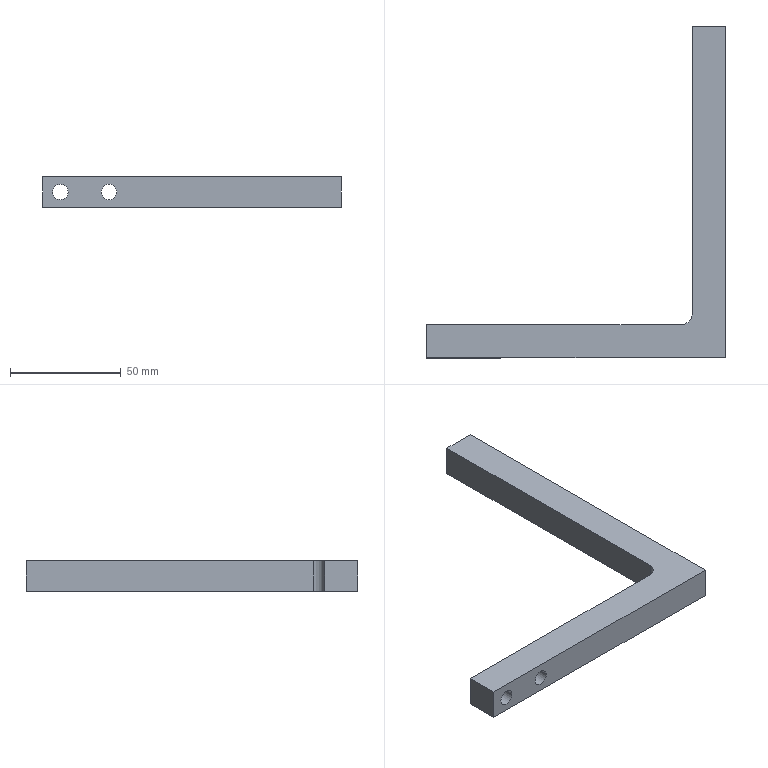Part | SolidWorks | features Extrusion 1, Fillet 1, ICE 1 | 1 solid | 13 faces | box 135 x 150 x 14 mm | volume 55621 mm3 | plane 8 | cylinder 5 | commonest cylinder face diameters 7 x4 10 x1
STEP:
#1=CARTESIAN_POINT('',(-130.5,0.,0.));
#2=VERTEX_POINT('',#1);
#3=CARTESIAN_POINT('',(-123.5,0.,0.));
#4=VERTEX_POINT('',#3);
#5=CARTESIAN_POINT('',(-127.,0.,0.));
#6=DIRECTION('',(0.,-1.,0.));
#7=DIRECTION('',(-1.,0.,0.));
#8=AXIS2_PLACEMENT_3D('',#5,#6,#7);
#9=CIRCLE('',#8,3.5);
#10=EDGE_CURVE('',#2,#4,#9,.T.);
#11=ORIENTED_EDGE('',*,*,#10,.T.);
#12=CARTESIAN_POINT('',(-123.5,15.,0.));
#13=VERTEX_POINT('',#12);
#14=CARTESIAN_POINT('',(-123.5,-0.001,0.));
#15=DIRECTION('',(0.,1.,0.));
#16=VECTOR('',#15,1000.);
#17=LINE('',#14,#16);
#18=EDGE_CURVE('',#4,#13,#17,.T.);
#19=ORIENTED_EDGE('',*,*,#18,.T.);
#20=CARTESIAN_POINT('',(-130.5,15.,0.));
#21=VERTEX_POINT('',#20);
#22=CARTESIAN_POINT('',(-127.,15.,0.));
#23=DIRECTION('',(0.,1.,0.));
#24=DIRECTION('',(-1.,0.,0.));
#25=AXIS2_PLACEMENT_3D('',#22,#23,#24);
#26=CIRCLE('',#25,3.5);
#27=EDGE_CURVE('',#13,#21,#26,.T.);
#28=ORIENTED_EDGE('',*,*,#27,.T.);
#29=CARTESIAN_POINT('',(-130.5,-0.001,0.));
#30=DIRECTION('',(0.,1.,0.));
#31=VECTOR('',#30,1000.);
#32=LINE('',#29,#31);
#33=EDGE_CURVE('',#2,#21,#32,.T.);
#34=ORIENTED_EDGE('',*,*,#33,.F.);
#35=EDGE_LOOP('',(#11,#19,#28,#34));
#36=FACE_OUTER_BOUND('',#35,.T.);
#37=CARTESIAN_POINT('',(-127.,-0.001,0.));
#38=DIRECTION('',(0.,1.,0.));
#39=DIRECTION('',(-1.,0.,0.));
#40=AXIS2_PLACEMENT_3D('',#37,#38,#39);
#41=CYLINDRICAL_SURFACE('',#40,3.5);
#42=ADVANCED_FACE('',(#36),#41,.F.);
#43=CARTESIAN_POINT('',(-108.5,0.,0.));
#44=VERTEX_POINT('',#43);
#45=CARTESIAN_POINT('',(-101.5,0.,0.));
#46=VERTEX_POINT('',#45);
#47=CARTESIAN_POINT('',(-105.,0.,0.));
#48=DIRECTION('',(0.,-1.,0.));
#49=DIRECTION('',(-1.,0.,0.));
#50=AXIS2_PLACEMENT_3D('',#47,#48,#49);
#51=CIRCLE('',#50,3.5);
#52=EDGE_CURVE('',#44,#46,#51,.T.);
#53=ORIENTED_EDGE('',*,*,#52,.T.);
#54=CARTESIAN_POINT('',(-101.5,15.,0.));
#55=VERTEX_POINT('',#54);
#56=CARTESIAN_POINT('',(-101.5,-0.001,0.));
#57=DIRECTION('',(0.,1.,0.));
#58=VECTOR('',#57,1000.);
#59=LINE('',#56,#58);
#60=EDGE_CURVE('',#46,#55,#59,.T.);
#61=ORIENTED_EDGE('',*,*,#60,.T.);
#62=CARTESIAN_POINT('',(-108.5,15.,0.));
#63=VERTEX_POINT('',#62);
#64=CARTESIAN_POINT('',(-105.,15.,0.));
#65=DIRECTION('',(0.,1.,0.));
#66=DIRECTION('',(-1.,0.,0.));
#67=AXIS2_PLACEMENT_3D('',#64,#65,#66);
#68=CIRCLE('',#67,3.5);
#69=EDGE_CURVE('',#55,#63,#68,.T.);
#70=ORIENTED_EDGE('',*,*,#69,.T.);
#71=CARTESIAN_POINT('',(-108.5,-0.001,0.));
#72=DIRECTION('',(0.,1.,0.));
#73=VECTOR('',#72,1000.);
#74=LINE('',#71,#73);
#75=EDGE_CURVE('',#44,#63,#74,.T.);
#76=ORIENTED_EDGE('',*,*,#75,.F.);
#77=EDGE_LOOP('',(#53,#61,#70,#76));
#78=FACE_OUTER_BOUND('',#77,.T.);
#79=CARTESIAN_POINT('',(-105.,-0.001,0.));
#80=DIRECTION('',(0.,1.,0.));
#81=DIRECTION('',(-1.,0.,0.));
#82=AXIS2_PLACEMENT_3D('',#79,#80,#81);
#83=CYLINDRICAL_SURFACE('',#82,3.5);
#84=ADVANCED_FACE('',(#78),#83,.F.);
#85=CARTESIAN_POINT('',(0.,0.,-7.));
#86=VERTEX_POINT('',#85);
#87=CARTESIAN_POINT('',(0.,150.,-7.));
#88=VERTEX_POINT('',#87);
#89=CARTESIAN_POINT('',(0.,150.,-7.));
#90=DIRECTION('',(0.,1.,0.));
#91=VECTOR('',#90,1000.);
#92=LINE('',#89,#91);
#93=EDGE_CURVE('',#86,#88,#92,.T.);
#94=ORIENTED_EDGE('',*,*,#93,.T.);
#95=CARTESIAN_POINT('',(0.,150.,7.));
#96=VERTEX_POINT('',#95);
#97=CARTESIAN_POINT('',(0.,150.,7.));
#98=DIRECTION('',(0.,0.,-1.));
#99=VECTOR('',#98,1000.);
#100=LINE('',#97,#99);
#101=EDGE_CURVE('',#96,#88,#100,.T.);
#102=ORIENTED_EDGE('',*,*,#101,.F.);
#103=CARTESIAN_POINT('',(0.,0.,7.));
#104=VERTEX_POINT('',#103);
#105=CARTESIAN_POINT('',(0.,150.,7.));
#106=DIRECTION('',(0.,1.,0.));
#107=VECTOR('',#106,1000.);
#108=LINE('',#105,#107);
#109=EDGE_CURVE('',#104,#96,#108,.T.);
#110=ORIENTED_EDGE('',*,*,#109,.F.);
#111=CARTESIAN_POINT('',(0.,0.,7.));
#112=DIRECTION('',(0.,0.,-1.));
#113=VECTOR('',#112,1000.);
#114=LINE('',#111,#113);
#115=EDGE_CURVE('',#104,#86,#114,.T.);
#116=ORIENTED_EDGE('',*,*,#115,.T.);
#117=EDGE_LOOP('',(#94,#102,#110,#116));
#118=FACE_OUTER_BOUND('',#117,.T.);
#119=CARTESIAN_POINT('',(0.,150.,7.));
#120=DIRECTION('',(-1.,0.,0.));
#121=DIRECTION('',(0.,-1.,0.));
#122=AXIS2_PLACEMENT_3D('',#119,#120,#121);
#123=PLANE('',#122);
#124=ADVANCED_FACE('',(#118),#123,.F.);
#125=CARTESIAN_POINT('',(-15.,150.,-7.));
#126=VERTEX_POINT('',#125);
#127=CARTESIAN_POINT('',(0.,150.,-7.));
#128=DIRECTION('',(-1.,0.,0.));
#129=VECTOR('',#128,1000.);
#130=LINE('',#127,#129);
#131=EDGE_CURVE('',#88,#126,#130,.T.);
#132=ORIENTED_EDGE('',*,*,#131,.T.);
#133=CARTESIAN_POINT('',(-15.,150.,7.));
#134=VERTEX_POINT('',#133);
#135=CARTESIAN_POINT('',(-15.,150.,7.));
#136=DIRECTION('',(0.,0.,-1.));
#137=VECTOR('',#136,1000.);
#138=LINE('',#135,#137);
#139=EDGE_CURVE('',#134,#126,#138,.T.);
#140=ORIENTED_EDGE('',*,*,#139,.F.);
#141=CARTESIAN_POINT('',(0.,150.,7.));
#142=DIRECTION('',(-1.,0.,0.));
#143=VECTOR('',#142,1000.);
#144=LINE('',#141,#143);
#145=EDGE_CURVE('',#96,#134,#144,.T.);
#146=ORIENTED_EDGE('',*,*,#145,.F.);
#147=ORIENTED_EDGE('',*,*,#101,.T.);
#148=EDGE_LOOP('',(#132,#140,#146,#147));
#149=FACE_OUTER_BOUND('',#148,.T.);
#150=CARTESIAN_POINT('',(0.,150.,7.));
#151=DIRECTION('',(0.,-1.,0.));
#152=DIRECTION('',(0.,0.,-1.));
#153=AXIS2_PLACEMENT_3D('',#150,#151,#152);
#154=PLANE('',#153);
#155=ADVANCED_FACE('',(#149),#154,.F.);
#156=CARTESIAN_POINT('',(-15.,20.,-7.));
#157=VERTEX_POINT('',#156);
#158=CARTESIAN_POINT('',(-15.,150.,-7.));
#159=DIRECTION('',(0.,-1.,0.));
#160=VECTOR('',#159,1000.);
#161=LINE('',#158,#160);
#162=EDGE_CURVE('',#126,#157,#161,.T.);
#163=ORIENTED_EDGE('',*,*,#162,.T.);
#164=CARTESIAN_POINT('',(-15.,20.,7.));
#165=VERTEX_POINT('',#164);
#166=CARTESIAN_POINT('',(-15.,20.,7.));
#167=DIRECTION('',(0.,0.,1.));
#168=VECTOR('',#167,1000.);
#169=LINE('',#166,#168);
#170=EDGE_CURVE('',#157,#165,#169,.T.);
#171=ORIENTED_EDGE('',*,*,#170,.T.);
#172=CARTESIAN_POINT('',(-15.,150.,7.));
#173=DIRECTION('',(0.,-1.,0.));
#174=VECTOR('',#173,1000.);
#175=LINE('',#172,#174);
#176=EDGE_CURVE('',#134,#165,#175,.T.);
#177=ORIENTED_EDGE('',*,*,#176,.F.);
#178=ORIENTED_EDGE('',*,*,#139,.T.);
#179=EDGE_LOOP('',(#163,#171,#177,#178));
#180=FACE_OUTER_BOUND('',#179,.T.);
#181=CARTESIAN_POINT('',(-15.,150.,7.));
#182=DIRECTION('',(1.,0.,0.));
#183=DIRECTION('',(0.,1.,0.));
#184=AXIS2_PLACEMENT_3D('',#181,#182,#183);
#185=PLANE('',#184);
#186=ADVANCED_FACE('',(#180),#185,.F.);
#187=CARTESIAN_POINT('',(-127.,15.,0.));
#188=DIRECTION('',(0.,1.,0.));
#189=DIRECTION('',(-1.,0.,0.));
#190=AXIS2_PLACEMENT_3D('',#187,#188,#189);
#191=CIRCLE('',#190,3.5);
#192=EDGE_CURVE('',#21,#13,#191,.T.);
#193=ORIENTED_EDGE('',*,*,#192,.F.);
#194=ORIENTED_EDGE('',*,*,#27,.F.);
#195=EDGE_LOOP('',(#193,#194));
#196=FACE_BOUND('',#195,.T.);
#197=CARTESIAN_POINT('',(-105.,15.,0.));
#198=DIRECTION('',(0.,1.,0.));
#199=DIRECTION('',(-1.,0.,0.));
#200=AXIS2_PLACEMENT_3D('',#197,#198,#199);
#201=CIRCLE('',#200,3.5);
#202=EDGE_CURVE('',#63,#55,#201,.T.);
#203=ORIENTED_EDGE('',*,*,#202,.F.);
#204=ORIENTED_EDGE('',*,*,#69,.F.);
#205=EDGE_LOOP('',(#203,#204));
#206=FACE_BOUND('',#205,.T.);
#207=CARTESIAN_POINT('',(-20.,15.,7.));
#208=VERTEX_POINT('',#207);
#209=CARTESIAN_POINT('',(-135.,15.,7.));
#210=VERTEX_POINT('',#209);
#211=CARTESIAN_POINT('',(-15.,15.,7.));
#212=DIRECTION('',(-1.,0.,0.));
#213=VECTOR('',#212,1000.);
#214=LINE('',#211,#213);
#215=EDGE_CURVE('',#208,#210,#214,.T.);
#216=ORIENTED_EDGE('',*,*,#215,.F.);
#217=CARTESIAN_POINT('',(-20.,15.,-7.));
#218=VERTEX_POINT('',#217);
#219=CARTESIAN_POINT('',(-20.,15.,-7.));
#220=DIRECTION('',(0.,0.,-1.));
#221=VECTOR('',#220,1000.);
#222=LINE('',#219,#221);
#223=EDGE_CURVE('',#208,#218,#222,.T.);
#224=ORIENTED_EDGE('',*,*,#223,.T.);
#225=CARTESIAN_POINT('',(-135.,15.,-7.));
#226=VERTEX_POINT('',#225);
#227=CARTESIAN_POINT('',(-15.,15.,-7.));
#228=DIRECTION('',(-1.,0.,0.));
#229=VECTOR('',#228,1000.);
#230=LINE('',#227,#229);
#231=EDGE_CURVE('',#218,#226,#230,.T.);
#232=ORIENTED_EDGE('',*,*,#231,.T.);
#233=CARTESIAN_POINT('',(-135.,15.,7.));
#234=DIRECTION('',(0.,0.,-1.));
#235=VECTOR('',#234,1000.);
#236=LINE('',#233,#235);
#237=EDGE_CURVE('',#210,#226,#236,.T.);
#238=ORIENTED_EDGE('',*,*,#237,.F.);
#239=EDGE_LOOP('',(#216,#224,#232,#238));
#240=FACE_OUTER_BOUND('',#239,.T.);
#241=CARTESIAN_POINT('',(-15.,15.,7.));
#242=DIRECTION('',(0.,-1.,0.));
#243=DIRECTION('',(1.,0.,0.));
#244=AXIS2_PLACEMENT_3D('',#241,#242,#243);
#245=PLANE('',#244);
#246=ADVANCED_FACE('',(#196,#206,#240),#245,.F.);
#247=CARTESIAN_POINT('',(-135.,0.,-7.));
#248=VERTEX_POINT('',#247);
#249=CARTESIAN_POINT('',(-135.,15.,-7.));
#250=DIRECTION('',(0.,-1.,0.));
#251=VECTOR('',#250,1000.);
#252=LINE('',#249,#251);
#253=EDGE_CURVE('',#226,#248,#252,.T.);
#254=ORIENTED_EDGE('',*,*,#253,.T.);
#255=CARTESIAN_POINT('',(-135.,0.,7.));
#256=VERTEX_POINT('',#255);
#257=CARTESIAN_POINT('',(-135.,0.,7.));
#258=DIRECTION('',(0.,0.,-1.));
#259=VECTOR('',#258,1000.);
#260=LINE('',#257,#259);
#261=EDGE_CURVE('',#256,#248,#260,.T.);
#262=ORIENTED_EDGE('',*,*,#261,.F.);
#263=CARTESIAN_POINT('',(-135.,15.,7.));
#264=DIRECTION('',(0.,-1.,0.));
#265=VECTOR('',#264,1000.);
#266=LINE('',#263,#265);
#267=EDGE_CURVE('',#210,#256,#266,.T.);
#268=ORIENTED_EDGE('',*,*,#267,.F.);
#269=ORIENTED_EDGE('',*,*,#237,.T.);
#270=EDGE_LOOP('',(#254,#262,#268,#269));
#271=FACE_OUTER_BOUND('',#270,.T.);
#272=CARTESIAN_POINT('',(-135.,15.,7.));
#273=DIRECTION('',(1.,0.,0.));
#274=DIRECTION('',(0.,0.,-1.));
#275=AXIS2_PLACEMENT_3D('',#272,#273,#274);
#276=PLANE('',#275);
#277=ADVANCED_FACE('',(#271),#276,.F.);
#278=ORIENTED_EDGE('',*,*,#10,.F.);
#279=CARTESIAN_POINT('',(-127.,0.,0.));
#280=DIRECTION('',(0.,-1.,0.));
#281=DIRECTION('',(-1.,0.,0.));
#282=AXIS2_PLACEMENT_3D('',#279,#280,#281);
#283=CIRCLE('',#282,3.5);
#284=EDGE_CURVE('',#4,#2,#283,.T.);
#285=ORIENTED_EDGE('',*,*,#284,.F.);
#286=EDGE_LOOP('',(#278,#285));
#287=FACE_BOUND('',#286,.T.);
#288=ORIENTED_EDGE('',*,*,#52,.F.);
#289=CARTESIAN_POINT('',(-105.,0.,0.));
#290=DIRECTION('',(0.,-1.,0.));
#291=DIRECTION('',(-1.,0.,0.));
#292=AXIS2_PLACEMENT_3D('',#289,#290,#291);
#293=CIRCLE('',#292,3.5);
#294=EDGE_CURVE('',#46,#44,#293,.T.);
#295=ORIENTED_EDGE('',*,*,#294,.F.);
#296=EDGE_LOOP('',(#288,#295));
#297=FACE_BOUND('',#296,.T.);
#298=CARTESIAN_POINT('',(0.,0.,-7.));
#299=DIRECTION('',(1.,0.,0.));
#300=VECTOR('',#299,1000.);
#301=LINE('',#298,#300);
#302=EDGE_CURVE('',#248,#86,#301,.T.);
#303=ORIENTED_EDGE('',*,*,#302,.T.);
#304=ORIENTED_EDGE('',*,*,#115,.F.);
#305=CARTESIAN_POINT('',(0.,0.,7.));
#306=DIRECTION('',(1.,0.,0.));
#307=VECTOR('',#306,1000.);
#308=LINE('',#305,#307);
#309=EDGE_CURVE('',#256,#104,#308,.T.);
#310=ORIENTED_EDGE('',*,*,#309,.F.);
#311=ORIENTED_EDGE('',*,*,#261,.T.);
#312=EDGE_LOOP('',(#303,#304,#310,#311));
#313=FACE_OUTER_BOUND('',#312,.T.);
#314=CARTESIAN_POINT('',(0.,0.,7.));
#315=DIRECTION('',(0.,1.,0.));
#316=DIRECTION('',(-1.,0.,0.));
#317=AXIS2_PLACEMENT_3D('',#314,#315,#316);
#318=PLANE('',#317);
#319=ADVANCED_FACE('',(#287,#297,#313),#318,.F.);
#320=ORIENTED_EDGE('',*,*,#109,.T.);
#321=ORIENTED_EDGE('',*,*,#145,.T.);
#322=ORIENTED_EDGE('',*,*,#176,.T.);
#323=CARTESIAN_POINT('',(-20.,20.,7.));
#324=DIRECTION('',(0.,0.,-1.));
#325=DIRECTION('',(-1.,0.,0.));
#326=AXIS2_PLACEMENT_3D('',#323,#324,#325);
#327=CIRCLE('',#326,5.);
#328=EDGE_CURVE('',#165,#208,#327,.T.);
#329=ORIENTED_EDGE('',*,*,#328,.T.);
#330=ORIENTED_EDGE('',*,*,#215,.T.);
#331=ORIENTED_EDGE('',*,*,#267,.T.);
#332=ORIENTED_EDGE('',*,*,#309,.T.);
#333=EDGE_LOOP('',(#320,#321,#322,#329,#330,#331,#332));
#334=FACE_OUTER_BOUND('',#333,.T.);
#335=CARTESIAN_POINT('',(0.,0.,7.));
#336=DIRECTION('',(0.,0.,-1.));
#337=DIRECTION('',(-1.,0.,0.));
#338=AXIS2_PLACEMENT_3D('',#335,#336,#337);
#339=PLANE('',#338);
#340=ADVANCED_FACE('',(#334),#339,.F.);
#341=ORIENTED_EDGE('',*,*,#93,.F.);
#342=ORIENTED_EDGE('',*,*,#302,.F.);
#343=ORIENTED_EDGE('',*,*,#253,.F.);
#344=ORIENTED_EDGE('',*,*,#231,.F.);
#345=CARTESIAN_POINT('',(-20.,20.,-7.));
#346=DIRECTION('',(0.,0.,1.));
#347=DIRECTION('',(-1.,0.,0.));
#348=AXIS2_PLACEMENT_3D('',#345,#346,#347);
#349=CIRCLE('',#348,5.);
#350=EDGE_CURVE('',#218,#157,#349,.T.);
#351=ORIENTED_EDGE('',*,*,#350,.T.);
#352=ORIENTED_EDGE('',*,*,#162,.F.);
#353=ORIENTED_EDGE('',*,*,#131,.F.);
#354=EDGE_LOOP('',(#341,#342,#343,#344,#351,#352,#353));
#355=FACE_OUTER_BOUND('',#354,.T.);
#356=CARTESIAN_POINT('',(0.,0.,-7.));
#357=DIRECTION('',(0.,0.,-1.));
#358=DIRECTION('',(-1.,0.,0.));
#359=AXIS2_PLACEMENT_3D('',#356,#357,#358);
#360=PLANE('',#359);
#361=ADVANCED_FACE('',(#355),#360,.T.);
#362=ORIENTED_EDGE('',*,*,#328,.F.);
#363=ORIENTED_EDGE('',*,*,#170,.F.);
#364=ORIENTED_EDGE('',*,*,#350,.F.);
#365=ORIENTED_EDGE('',*,*,#223,.F.);
#366=EDGE_LOOP('',(#362,#363,#364,#365));
#367=FACE_OUTER_BOUND('',#366,.T.);
#368=CARTESIAN_POINT('',(-20.,20.,7.));
#369=DIRECTION('',(0.,0.,1.));
#370=DIRECTION('',(1.,0.,0.));
#371=AXIS2_PLACEMENT_3D('',#368,#369,#370);
#372=CYLINDRICAL_SURFACE('',#371,5.);
#373=ADVANCED_FACE('',(#367),#372,.F.);
#374=ORIENTED_EDGE('',*,*,#60,.F.);
#375=ORIENTED_EDGE('',*,*,#294,.T.);
#376=ORIENTED_EDGE('',*,*,#75,.T.);
#377=ORIENTED_EDGE('',*,*,#202,.T.);
#378=EDGE_LOOP('',(#374,#375,#376,#377));
#379=FACE_OUTER_BOUND('',#378,.T.);
#380=CARTESIAN_POINT('',(-105.,-0.001,0.));
#381=DIRECTION('',(0.,1.,0.));
#382=DIRECTION('',(-1.,0.,0.));
#383=AXIS2_PLACEMENT_3D('',#380,#381,#382);
#384=CYLINDRICAL_SURFACE('',#383,3.5);
#385=ADVANCED_FACE('',(#379),#384,.F.);
#386=ORIENTED_EDGE('',*,*,#18,.F.);
#387=ORIENTED_EDGE('',*,*,#284,.T.);
#388=ORIENTED_EDGE('',*,*,#33,.T.);
#389=ORIENTED_EDGE('',*,*,#192,.T.);
#390=EDGE_LOOP('',(#386,#387,#388,#389));
#391=FACE_OUTER_BOUND('',#390,.T.);
#392=CARTESIAN_POINT('',(-127.,-0.001,0.));
#393=DIRECTION('',(0.,1.,0.));
#394=DIRECTION('',(-1.,0.,0.));
#395=AXIS2_PLACEMENT_3D('',#392,#393,#394);
#396=CYLINDRICAL_SURFACE('',#395,3.5);
#397=ADVANCED_FACE('',(#391),#396,.F.);
#398=CLOSED_SHELL('',(#42,#84,#124,#155,#186,#246,#277,#319,#340,#361,#373,#385,#397));
#399=MANIFOLD_SOLID_BREP('',#398);
#400=CARTESIAN_POINT('',(0.,0.,0.));
#401=DIRECTION('',(0.,0.,1.));
#402=DIRECTION('',(1.,0.,0.));
#403=AXIS2_PLACEMENT_3D('',#400,#401,#402);
#404=(LENGTH_UNIT()NAMED_UNIT(*)SI_UNIT(.MILLI.,.METRE.));
#405=UNCERTAINTY_MEASURE_WITH_UNIT(LENGTH_MEASURE(0.00001),#404,'','');
#406=(NAMED_UNIT(*)PLANE_ANGLE_UNIT()SI_UNIT($,.RADIAN.));
#407=(NAMED_UNIT(*)SI_UNIT($,.STERADIAN.)SOLID_ANGLE_UNIT());
#408=(GEOMETRIC_REPRESENTATION_CONTEXT(3)GLOBAL_UNCERTAINTY_ASSIGNED_CONTEXT((#405))GLOBAL_UNIT_ASSIGNED_CONTEXT((#404,#406,#407))REPRESENTATION_CONTEXT('',''));
#409=ADVANCED_BREP_SHAPE_REPRESENTATION('',(#399,#403),#408);